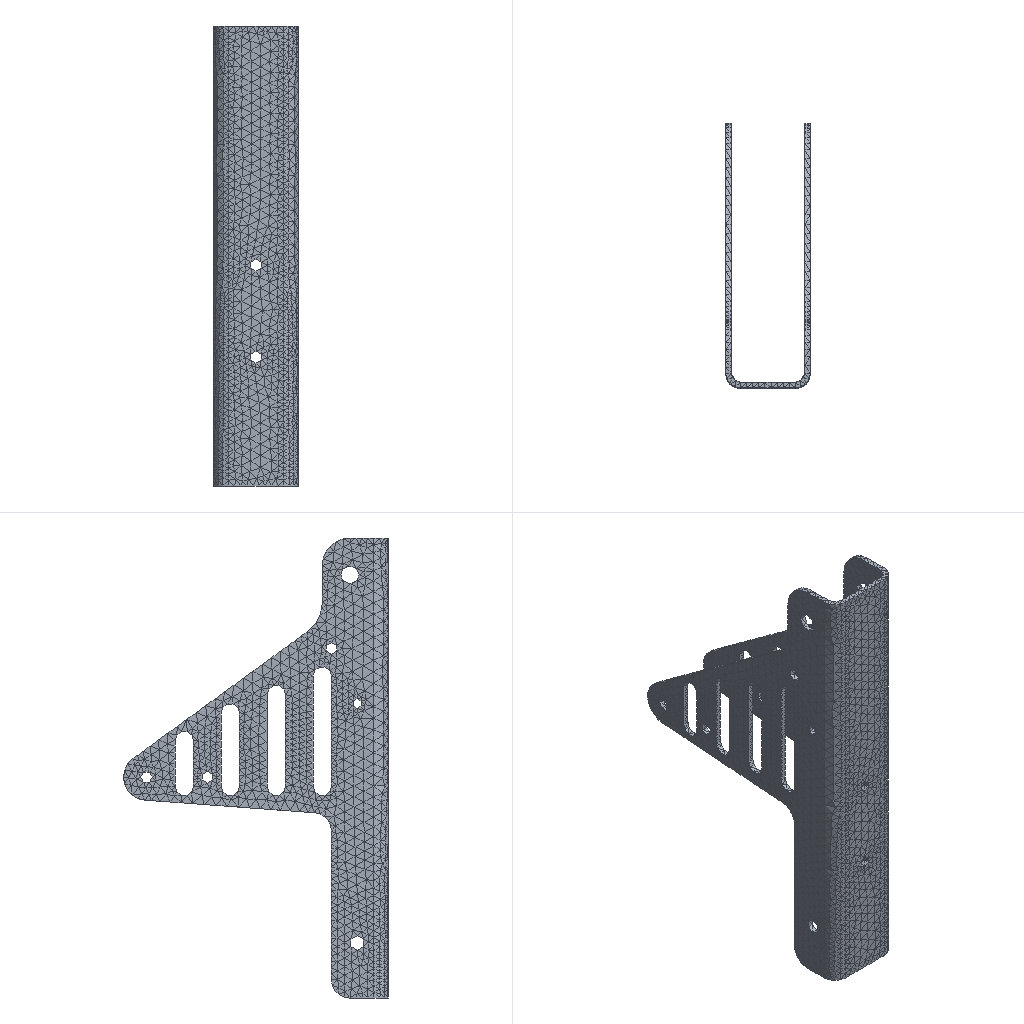Simulation study | nx simcenter
Set-up summary:
category,name,step,type,value,unit,region
solver,nx_nastran (Simcenter)
units,not stated in the deck,,not stated
analysis,deck,,static,static
analysis,solution,,SOL,101
load_step,SUBCASE 1,1,SUBCASE,SPC=1 LOAD=2
load_step,requested,,,1
mesh,nodes,,,27273
mesh,elements,,,12785
element_type,CTETRA,,solid,12785
load,nodal force total,,FX,0.0,model units
load,nodal force total,,FY,0.0,model units
load,nodal force total,,FZ,0.0,model units
load,load commands in deck,,count,5124
bc,support commands in deck,,count,1943
analysis,NX solution 0,,Structural,SESTATIC 101 - Single Constraint
check,setup vs results,,match,every grid point's frame and coordinates and every element id; grid points of CTETRA elements
Nastran input file, long lists of numbers shortened:
$*$$$$$$$$$$$$$$$$$$$$$$$$$$$$$$$$$$$$$$$$$$$$$$$$$$$$$$$$$$$$$$$$$
$*
$*                    Simcenter v12.0.0.27 Translator
$*                    for NX Nastran version 12.0
$ (40 more lines like these left out)
ID,NASTRAN,支撑架_fem1_sim1-solution_1
SOL 101
CEND
$*
$*$$$$$$$$$$$$$$$$$$$$$$$$$$$$$$$$$$$
$*
$* CASE CONTROL
$*
$*$$$$$$$$$$$$$$$$$$$$$$$$$$$$$$$$$$$
$*
ECHO = NONE
SPC = 1
OUTPUT
DISPLACEMENT(PLOT,REAL) = ALL
SPCFORCES(PLOT,REAL) = ALL
STRESS(PLOT,REAL,VONMISES,CENTER) = ALL
$*  Step: Subcase - Static Loads 1
SUBCASE 1
  LABEL = Subcase - Static Loads 1
  LOAD = 2
$*
$*$$$$$$$$$$$$$$$$$$$$$$$$$$$$$$$$$$$
$*
$* BULK DATA
$*
$*$$$$$$$$$$$$$$$$$$$$$$$$$$$$$$$$$$$
$*
BEGIN BULK
$*
$* PARAM CARDS
$*
PARAM      K6ROT100.0000
PARAM     OIBULK     YES
PARAM    OMACHPR     YES
PARAM       POST      -2
PARAM    POSTEXT     YES
PARAM    UNITSYS   MN-MM
$*
$* GRID CARDS
$*
GRID*                  1               0-2.157066931E+014.7059468680E+01+
*       -7.495982798E+01               0
GRID*                  2               02.1444292690E+01-4.250513096E+00+
*       -4.142397048E+01               0
$ (54542 more lines like these left out)
$*
$* ELEMENT CARDS
$*
$*  Mesh Collector: Solid(1)
$*  Mesh: 3d_mesh(1)
CTETRA         1       1   17846   21490   21491   21494      30   22108+
+             31      32   22091   22107
CTETRA         2       1   17849   17852   17850   21497   18303   18305+
+          18304      33      34      35
$ (25566 more lines like these left out)
$*
$* PROPERTY CARDS
$*
$*  Property: PSOLID1
PSOLID         1       1       0                           SMECH
$*
$* MATERIAL CARDS
$*
$* Material: AISI_310_SS::support bracket_fem1::[1]
MAT1           11.9314+8        0.3000007.9278-61.4750-5
MATT1          1       1               2               3
TABLEM1        1                       1                                +
+        20.00001.9314+8 21.11001.9314+8    ENDT
TABLEM1        2                       1                                +
+        20.00000.300000 21.11000.300000    ENDT
TABLEM1        3                       1                                +
+        20.00001.4750-5 93.33001.5120-5107.22001.5192-5121.11001.5264-5+
+       135.00001.5336-5148.89001.5390-5162.78001.5462-5176.67001.5534-5+
+       190.56001.5588-5204.44001.5660-5218.33001.5732-5232.22001.5786-5+
+       246.11001.5840-5260.00001.5912-5273.89001.5966-5287.78001.6020-5+
+       301.67001.6092-5315.56001.6146-5329.44001.6200-5343.33001.6254-5+
+       357.22001.6326-5371.11001.6380-5385.00001.6434-5398.89001.6506-5+
+       412.78001.6560-5426.67001.6614-5440.56001.6668-5454.44001.6740-5+
+       468.33001.6794-5482.22001.6848-5496.11001.6920-5510.00001.6974-5+
+       523.89001.7028-5537.78001.7100-5551.67001.7172-5565.56001.7226-5+
+       579.44001.7298-5593.33001.7370-5607.22001.7442-5621.11001.7514-5+
+       635.00001.7586-5648.89001.7640-5662.78001.7694-5676.67001.7766-5+
+       690.56001.7820-5704.44001.7874-5718.33001.7928-5732.22001.7982-5+
+       746.11001.8036-5760.00001.8090-5773.89001.8144-5787.78001.8198-5+
+       801.67001.8252-5815.56001.8324-5829.44001.8378-5843.33001.8432-5+
+       857.22001.8486-5871.11001.8540-5885.00001.8594-5898.89001.8648-5+
+       912.78001.8702-5926.67001.8756-5940.56001.8810-5954.44001.8846-5+
+       968.33001.8900-5982.22001.8954-5    ENDT
$*
$* LOAD AND CONSTRAINT CARDS
$*
$*  Constraint: NoTrans(1)
SPC            1   14226     123  0.0000
SPC            1   14227     123  0.0000
SPC            1   14228     123  0.0000
SPC            1   14229     123  0.0000
$ (1939 more lines like these left out)
$*  Load: Pressure(1)
PLOAD4         2       1 3000.00                           21490   17846
PLOAD4         2       2 3000.00                           17849   21497
PLOAD4         2       3 3000.00                           17849   21494
PLOAD4         2       4 3000.00                           27244   27206
$ (5120 more lines like these left out)
ENDDATA d71dda7d
Results summary:
result,analysis,,,static
result,last_loadstep,,,1
result,primary field,,,displacements
result,max displacement,,,0.03694,model units
result,reaction total,,FX,1414.809,model units
result,reaction total,,FY,0.007202,model units
result,reaction total,,FZ,0.01611,model units
result,NX solution 0,,loadcases,1,mm